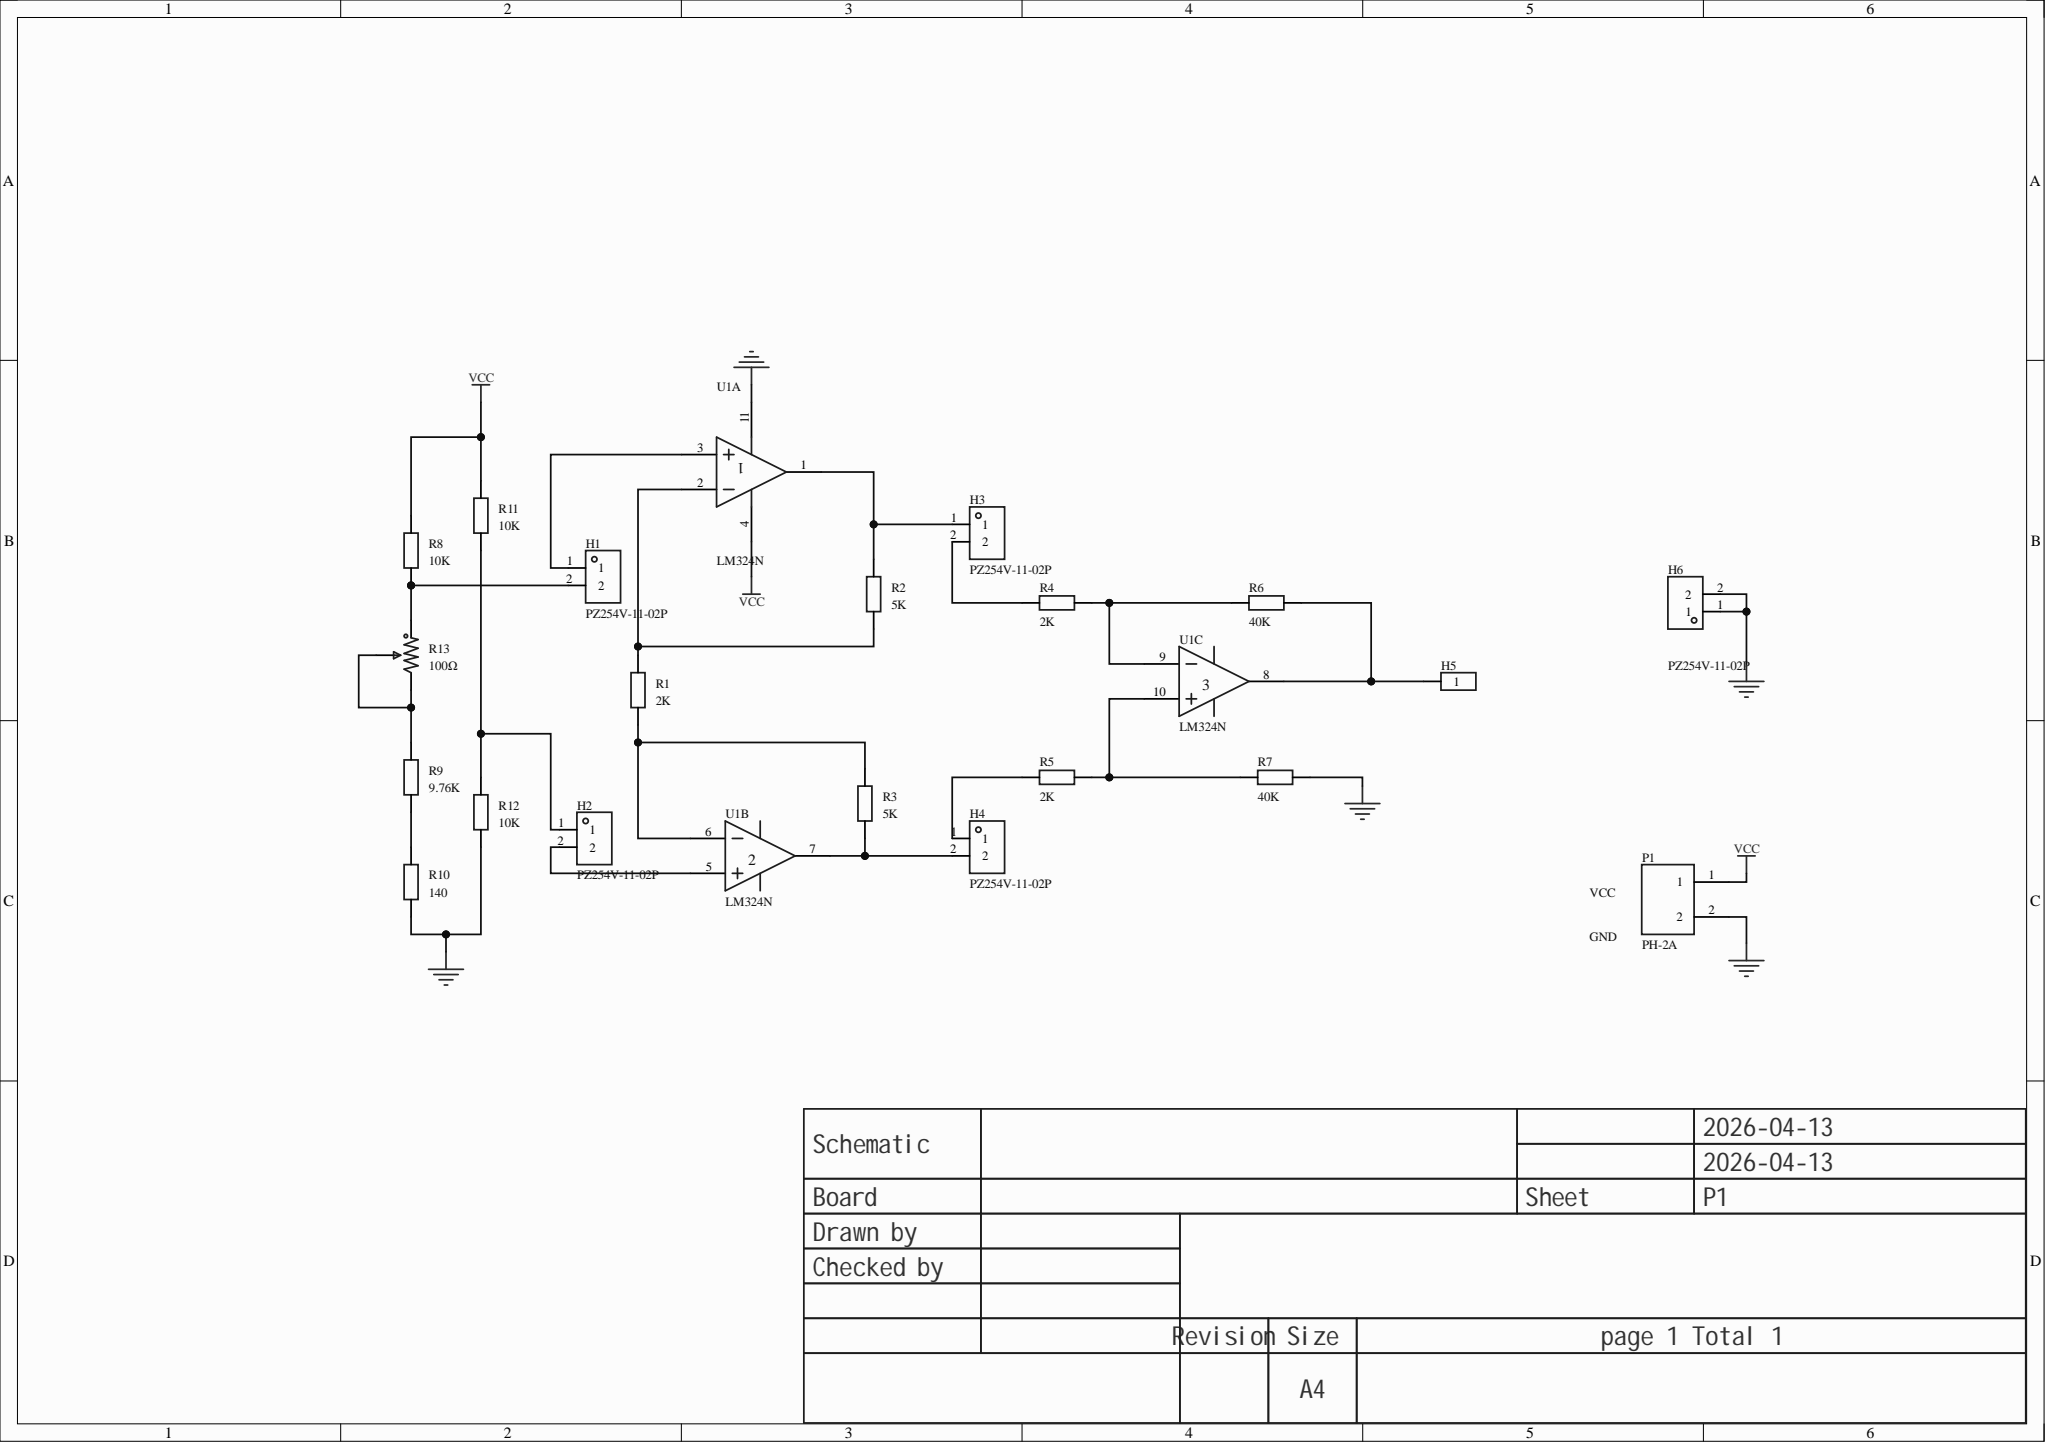Circuit board | Altium Designer | 21 parts | 17 nets
Bill of materials:
Comment,Description,Designator,Footprint,LibRef,Quantity
"PZ254V-11-02P","Pin structure:1x2P;Pitch:2.54mm;Row spacing:-;Round/square pins:Square;Mounting:Through-hole;Rows:Single row;Total pins:2P;Rated current:3A;Rated voltage:250V;Mating pin length:6mm;Body height:2.5mm;Tail length:3mm;Contact material:Brass;Contact plating:-;Operating temperature:-40℃~+105℃;Color:Black;","H1, H2, H3, H4, H6","HDR-TH_2P-P2.54-V-M","PZ254V-11-02P","5"
"","","H5","HDR-TH_1P-V-M_XKB_X4611WV-01I-C28D40","HDR-M_2.54_1x1P","1"
"PH-2A","Reference series:PH;Pitch:2mm;Pin structure:1x2P;Rows:1;Pins per row:2;Row spacing:-;Mounting:-;Contact material:-;","P1","CONN-TH_2P-P2.00_PH-2A_C2319","PH-2A","1"
"2K","","R1, R4, R5","R0805_1","Res_0603","3"
"5K","","R2, R3","R0805_1","Res_0603","2"
"40K","","R6, R7","R0805_1","Res_0603","2"
"10K","","R8, R11, R12","R0805_1","Res_0603","3"
"9.76K","","R9","R0805_1","Res_0603","1"
"140","","R10","R0805_1","Res_0603","1"
"100Ω","Resistance:100Ω;Tolerance:±10%;Power:500mW;Temperature coefficient:±250ppm/?;","R13","RES-ADJ-TH_3296W","3296W-1-101_C48997939","1"
"LM324N","Amplifier count:Quad;Rail-to-rail:-;Gain bandwidth product (GBP):-;Input offset voltage (Vos):9mV;Slew rate (SR):-;Input bias current (Ib):250nA;","U1","DIP-14_L19.4-W6.4-P2.54-LS7.6-BL","LM324N_C725320","1"
Netlist (Protel format):
[
H1
HDR-TH_2P-P2.54-V-M
PZ254V-11-02P



]
[
H2
HDR-TH_2P-P2.54-V-M
PZ254V-11-02P



]
[
H3
HDR-TH_2P-P2.54-V-M
PZ254V-11-02P



]
[
H4
HDR-TH_2P-P2.54-V-M
PZ254V-11-02P



]
[
H5
HDR-TH_1P-V-M_XKB_X4611WV-01I-C28D40




]
[
H6
HDR-TH_2P-P2.54-V-M
PZ254V-11-02P



]
[
P1
CONN-TH_2P-P2.00_PH-2A_C2319
PH-2A



]
[
R1
R0805_1
2K



]
[
R2
R0805_1
5K



]
[
R3
R0805_1
5K



]
[
R4
R0805_1
2K



]
[
R5
R0805_1
2K



]
[
R6
R0805_1
40K



]
[
R7
R0805_1
40K



]
[
R8
R0805_1
10K



]
[
R9
R0805_1
9.76K



]
[
R10
R0805_1
140



]
[
R11
R0805_1
10K



]
[
R12
R0805_1
10K



]
[
R13
RES-ADJ-TH_3296W
100Ω



]
[
U1
DIP-14_L19.4-W6.4-P2.54-LS7.6-BL
LM324N



]
(
VCC
P1-1
R8-2
R11-2
U1-4
)
(
NetR9_2
R9-2
R13-2
R13-3
)
(
NetR9_1
R9-1
R10-2
)
(
NetR5_1
R5-1
R7-2
U1-10
)
(
NetR4_1
R4-1
R6-2
U1-9
)
(
NetR1_2
R1-2
R2-1
U1-2
)
(
NetR1_1
R1-1
R3-2
U1-6
)
(
NetH5_1
H5-1
R6-1
U1-8
)
(
NetH4_2
H4-2
R3-1
U1-7
)
(
NetH4_1
H4-1
R5-2
)
(
NetH3_2
H3-2
R4-2
)
(
NetH3_1
H3-1
R2-2
U1-1
)
(
NetH2_2
H2-2
U1-5
)
(
NetH2_1
H2-1
R11-1
R12-2
)
(
NetH1_2
H1-2
R8-1
R13-1
)
(
NetH1_1
H1-1
U1-3
)
(
GND
H6-1
H6-2
P1-2
R7-1
R10-1
R12-1
U1-11
)